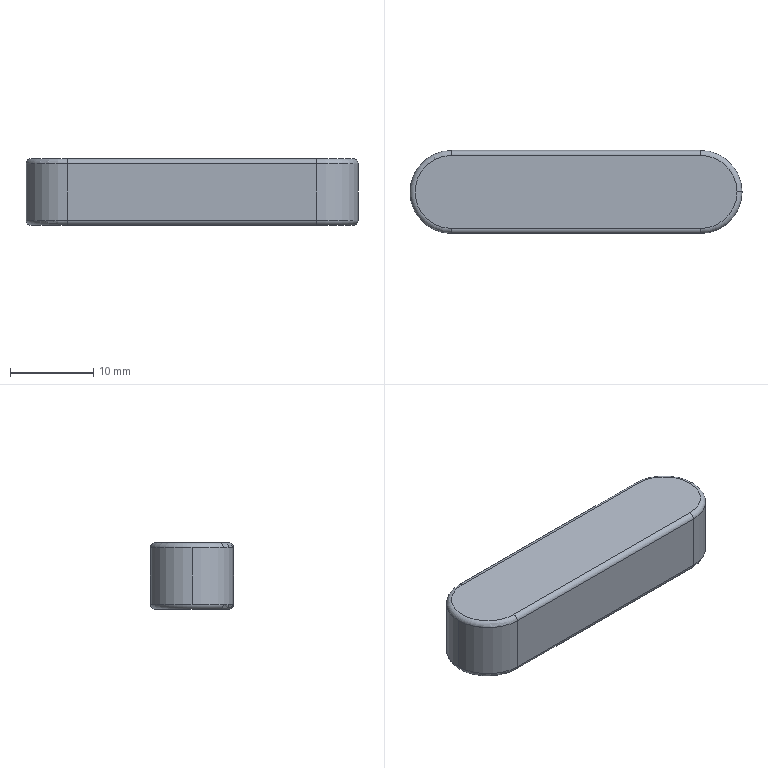Part | SolidWorks | features Extrusion 1, Fillet 1 | 1 solid | 17 faces | box 40 x 10 x 8 mm | volume 3014 mm3 | cylinder 7 | torus 6 | plane 4 | commonest cylinder face diameters 1.2 x4 10 x3
STEP:
#1=CARTESIAN_POINT('',(19.4,0.,0.));
#2=VERTEX_POINT('',#1);
#3=CARTESIAN_POINT('',(15.,-4.4,0.));
#4=VERTEX_POINT('',#3);
#5=CARTESIAN_POINT('',(15.,0.,0.));
#6=DIRECTION('',(0.,0.,-1.));
#7=DIRECTION('',(1.,0.,0.));
#8=AXIS2_PLACEMENT_3D('',#5,#6,#7);
#9=CIRCLE('',#8,4.4);
#10=EDGE_CURVE('',#2,#4,#9,.T.);
#11=ORIENTED_EDGE('',*,*,#10,.F.);
#12=CARTESIAN_POINT('',(20.,0.,0.6));
#13=VERTEX_POINT('',#12);
#14=CARTESIAN_POINT('',(19.4,0.,0.6));
#15=DIRECTION('',(0.,-1.,0.));
#16=DIRECTION('',(0.,0.,-1.));
#17=AXIS2_PLACEMENT_3D('',#14,#15,#16);
#18=CIRCLE('',#17,0.6);
#19=EDGE_CURVE('',#2,#13,#18,.T.);
#20=ORIENTED_EDGE('',*,*,#19,.T.);
#21=CARTESIAN_POINT('',(15.,-5.,0.6));
#22=VERTEX_POINT('',#21);
#23=CARTESIAN_POINT('',(15.,0.,0.6));
#24=DIRECTION('',(0.,0.,1.));
#25=DIRECTION('',(1.,0.,0.));
#26=AXIS2_PLACEMENT_3D('',#23,#24,#25);
#27=CIRCLE('',#26,5.);
#28=EDGE_CURVE('',#22,#13,#27,.T.);
#29=ORIENTED_EDGE('',*,*,#28,.F.);
#30=CARTESIAN_POINT('',(15.,-4.4,0.6));
#31=DIRECTION('',(1.,0.,0.));
#32=DIRECTION('',(0.,0.,-1.));
#33=AXIS2_PLACEMENT_3D('',#30,#31,#32);
#34=CIRCLE('',#33,0.6);
#35=EDGE_CURVE('',#22,#4,#34,.T.);
#36=ORIENTED_EDGE('',*,*,#35,.T.);
#37=EDGE_LOOP('',(#11,#20,#29,#36));
#38=FACE_OUTER_BOUND('',#37,.T.);
#39=CARTESIAN_POINT('',(15.,0.,0.6));
#40=DIRECTION('',(0.,0.,1.));
#41=DIRECTION('',(1.,0.,0.));
#42=AXIS2_PLACEMENT_3D('',#39,#40,#41);
#43=TOROIDAL_SURFACE('',#42,4.4,0.6);
#44=ADVANCED_FACE('',(#38),#43,.T.);
#45=CARTESIAN_POINT('',(20.,0.,7.4));
#46=VERTEX_POINT('',#45);
#47=CARTESIAN_POINT('',(15.,-5.,7.4));
#48=VERTEX_POINT('',#47);
#49=CARTESIAN_POINT('',(15.,0.,7.4));
#50=DIRECTION('',(0.,0.,-1.));
#51=DIRECTION('',(1.,0.,0.));
#52=AXIS2_PLACEMENT_3D('',#49,#50,#51);
#53=CIRCLE('',#52,5.);
#54=EDGE_CURVE('',#46,#48,#53,.T.);
#55=ORIENTED_EDGE('',*,*,#54,.F.);
#56=CARTESIAN_POINT('',(19.4,0.,8.));
#57=VERTEX_POINT('',#56);
#58=CARTESIAN_POINT('',(19.4,0.,7.4));
#59=DIRECTION('',(0.,-1.,0.));
#60=DIRECTION('',(0.,0.,-1.));
#61=AXIS2_PLACEMENT_3D('',#58,#59,#60);
#62=CIRCLE('',#61,0.6);
#63=EDGE_CURVE('',#46,#57,#62,.T.);
#64=ORIENTED_EDGE('',*,*,#63,.T.);
#65=CARTESIAN_POINT('',(15.,-4.4,8.));
#66=VERTEX_POINT('',#65);
#67=CARTESIAN_POINT('',(15.,0.,8.));
#68=DIRECTION('',(0.,0.,1.));
#69=DIRECTION('',(1.,0.,0.));
#70=AXIS2_PLACEMENT_3D('',#67,#68,#69);
#71=CIRCLE('',#70,4.4);
#72=EDGE_CURVE('',#66,#57,#71,.T.);
#73=ORIENTED_EDGE('',*,*,#72,.F.);
#74=CARTESIAN_POINT('',(15.,-4.4,7.4));
#75=DIRECTION('',(1.,0.,0.));
#76=DIRECTION('',(0.,0.,-1.));
#77=AXIS2_PLACEMENT_3D('',#74,#75,#76);
#78=CIRCLE('',#77,0.6);
#79=EDGE_CURVE('',#66,#48,#78,.T.);
#80=ORIENTED_EDGE('',*,*,#79,.T.);
#81=EDGE_LOOP('',(#55,#64,#73,#80));
#82=FACE_OUTER_BOUND('',#81,.T.);
#83=CARTESIAN_POINT('',(15.,0.,7.4));
#84=DIRECTION('',(0.,0.,1.));
#85=DIRECTION('',(1.,0.,0.));
#86=AXIS2_PLACEMENT_3D('',#83,#84,#85);
#87=TOROIDAL_SURFACE('',#86,4.4,0.6);
#88=ADVANCED_FACE('',(#82),#87,.T.);
#89=CARTESIAN_POINT('',(-15.,-5.,7.4));
#90=VERTEX_POINT('',#89);
#91=CARTESIAN_POINT('',(-20.,0.,7.4));
#92=VERTEX_POINT('',#91);
#93=CARTESIAN_POINT('',(-15.,0.,7.4));
#94=DIRECTION('',(0.,0.,-1.));
#95=DIRECTION('',(1.,0.,0.));
#96=AXIS2_PLACEMENT_3D('',#93,#94,#95);
#97=CIRCLE('',#96,5.);
#98=EDGE_CURVE('',#90,#92,#97,.T.);
#99=ORIENTED_EDGE('',*,*,#98,.T.);
#100=CARTESIAN_POINT('',(-20.,0.,0.6));
#101=VERTEX_POINT('',#100);
#102=CARTESIAN_POINT('',(-20.,0.,8.));
#103=DIRECTION('',(0.,0.,-1.));
#104=VECTOR('',#103,1000.);
#105=LINE('',#102,#104);
#106=EDGE_CURVE('',#92,#101,#105,.T.);
#107=ORIENTED_EDGE('',*,*,#106,.T.);
#108=CARTESIAN_POINT('',(-15.,-5.,0.6));
#109=VERTEX_POINT('',#108);
#110=CARTESIAN_POINT('',(-15.,0.,0.6));
#111=DIRECTION('',(0.,0.,1.));
#112=DIRECTION('',(1.,0.,0.));
#113=AXIS2_PLACEMENT_3D('',#110,#111,#112);
#114=CIRCLE('',#113,5.);
#115=EDGE_CURVE('',#101,#109,#114,.T.);
#116=ORIENTED_EDGE('',*,*,#115,.T.);
#117=CARTESIAN_POINT('',(-15.,-5.,8.));
#118=DIRECTION('',(0.,0.,-1.));
#119=VECTOR('',#118,1000.);
#120=LINE('',#117,#119);
#121=EDGE_CURVE('',#90,#109,#120,.T.);
#122=ORIENTED_EDGE('',*,*,#121,.F.);
#123=EDGE_LOOP('',(#99,#107,#116,#122));
#124=FACE_OUTER_BOUND('',#123,.T.);
#125=CARTESIAN_POINT('',(-15.,0.,8.));
#126=DIRECTION('',(0.,0.,-1.));
#127=DIRECTION('',(-1.,0.,0.));
#128=AXIS2_PLACEMENT_3D('',#125,#126,#127);
#129=CYLINDRICAL_SURFACE('',#128,5.);
#130=ADVANCED_FACE('',(#124),#129,.T.);
#131=ORIENTED_EDGE('',*,*,#106,.F.);
#132=CARTESIAN_POINT('',(-15.,5.,7.4));
#133=VERTEX_POINT('',#132);
#134=CARTESIAN_POINT('',(-15.,0.,7.4));
#135=DIRECTION('',(0.,0.,-1.));
#136=DIRECTION('',(1.,0.,0.));
#137=AXIS2_PLACEMENT_3D('',#134,#135,#136);
#138=CIRCLE('',#137,5.);
#139=EDGE_CURVE('',#92,#133,#138,.T.);
#140=ORIENTED_EDGE('',*,*,#139,.T.);
#141=CARTESIAN_POINT('',(-15.,5.,0.6));
#142=VERTEX_POINT('',#141);
#143=CARTESIAN_POINT('',(-15.,5.,8.));
#144=DIRECTION('',(0.,0.,-1.));
#145=VECTOR('',#144,1000.);
#146=LINE('',#143,#145);
#147=EDGE_CURVE('',#133,#142,#146,.T.);
#148=ORIENTED_EDGE('',*,*,#147,.T.);
#149=CARTESIAN_POINT('',(-15.,0.,0.6));
#150=DIRECTION('',(0.,0.,1.));
#151=DIRECTION('',(1.,0.,0.));
#152=AXIS2_PLACEMENT_3D('',#149,#150,#151);
#153=CIRCLE('',#152,5.);
#154=EDGE_CURVE('',#142,#101,#153,.T.);
#155=ORIENTED_EDGE('',*,*,#154,.T.);
#156=EDGE_LOOP('',(#131,#140,#148,#155));
#157=FACE_OUTER_BOUND('',#156,.T.);
#158=CARTESIAN_POINT('',(-15.,0.,8.));
#159=DIRECTION('',(0.,0.,-1.));
#160=DIRECTION('',(-1.,0.,0.));
#161=AXIS2_PLACEMENT_3D('',#158,#159,#160);
#162=CYLINDRICAL_SURFACE('',#161,5.);
#163=ADVANCED_FACE('',(#157),#162,.T.);
#164=CARTESIAN_POINT('',(15.,-5.,8.));
#165=DIRECTION('',(0.,0.,-1.));
#166=VECTOR('',#165,1000.);
#167=LINE('',#164,#166);
#168=EDGE_CURVE('',#48,#22,#167,.T.);
#169=ORIENTED_EDGE('',*,*,#168,.F.);
#170=CARTESIAN_POINT('',(-15.,-5.,7.4));
#171=DIRECTION('',(-1.,0.,0.));
#172=VECTOR('',#171,1000.);
#173=LINE('',#170,#172);
#174=EDGE_CURVE('',#48,#90,#173,.T.);
#175=ORIENTED_EDGE('',*,*,#174,.T.);
#176=ORIENTED_EDGE('',*,*,#121,.T.);
#177=CARTESIAN_POINT('',(-15.,-5.,0.6));
#178=DIRECTION('',(1.,0.,0.));
#179=VECTOR('',#178,1000.);
#180=LINE('',#177,#179);
#181=EDGE_CURVE('',#109,#22,#180,.T.);
#182=ORIENTED_EDGE('',*,*,#181,.T.);
#183=EDGE_LOOP('',(#169,#175,#176,#182));
#184=FACE_OUTER_BOUND('',#183,.T.);
#185=CARTESIAN_POINT('',(-15.,-5.,8.));
#186=DIRECTION('',(0.,1.,0.));
#187=DIRECTION('',(-1.,0.,0.));
#188=AXIS2_PLACEMENT_3D('',#185,#186,#187);
#189=PLANE('',#188);
#190=ADVANCED_FACE('',(#184),#189,.F.);
#191=CARTESIAN_POINT('',(15.,5.,7.4));
#192=VERTEX_POINT('',#191);
#193=CARTESIAN_POINT('',(15.,5.,0.6));
#194=VERTEX_POINT('',#193);
#195=CARTESIAN_POINT('',(15.,5.,8.));
#196=DIRECTION('',(0.,0.,-1.));
#197=VECTOR('',#196,1000.);
#198=LINE('',#195,#197);
#199=EDGE_CURVE('',#192,#194,#198,.T.);
#200=ORIENTED_EDGE('',*,*,#199,.F.);
#201=CARTESIAN_POINT('',(15.,0.,7.4));
#202=DIRECTION('',(0.,0.,-1.));
#203=DIRECTION('',(1.,0.,0.));
#204=AXIS2_PLACEMENT_3D('',#201,#202,#203);
#205=CIRCLE('',#204,5.);
#206=EDGE_CURVE('',#192,#46,#205,.T.);
#207=ORIENTED_EDGE('',*,*,#206,.T.);
#208=ORIENTED_EDGE('',*,*,#54,.T.);
#209=ORIENTED_EDGE('',*,*,#168,.T.);
#210=ORIENTED_EDGE('',*,*,#28,.T.);
#211=CARTESIAN_POINT('',(15.,0.,0.6));
#212=DIRECTION('',(0.,0.,1.));
#213=DIRECTION('',(1.,0.,0.));
#214=AXIS2_PLACEMENT_3D('',#211,#212,#213);
#215=CIRCLE('',#214,5.);
#216=EDGE_CURVE('',#13,#194,#215,.T.);
#217=ORIENTED_EDGE('',*,*,#216,.T.);
#218=EDGE_LOOP('',(#200,#207,#208,#209,#210,#217));
#219=FACE_OUTER_BOUND('',#218,.T.);
#220=CARTESIAN_POINT('',(15.,0.,8.));
#221=DIRECTION('',(0.,0.,-1.));
#222=DIRECTION('',(-1.,0.,0.));
#223=AXIS2_PLACEMENT_3D('',#220,#221,#222);
#224=CYLINDRICAL_SURFACE('',#223,5.);
#225=ADVANCED_FACE('',(#219),#224,.T.);
#226=ORIENTED_EDGE('',*,*,#147,.F.);
#227=CARTESIAN_POINT('',(15.,5.,7.4));
#228=DIRECTION('',(1.,0.,0.));
#229=VECTOR('',#228,1000.);
#230=LINE('',#227,#229);
#231=EDGE_CURVE('',#133,#192,#230,.T.);
#232=ORIENTED_EDGE('',*,*,#231,.T.);
#233=ORIENTED_EDGE('',*,*,#199,.T.);
#234=CARTESIAN_POINT('',(-15.,5.,0.6));
#235=DIRECTION('',(-1.,0.,0.));
#236=VECTOR('',#235,1000.);
#237=LINE('',#234,#236);
#238=EDGE_CURVE('',#194,#142,#237,.T.);
#239=ORIENTED_EDGE('',*,*,#238,.T.);
#240=EDGE_LOOP('',(#226,#232,#233,#239));
#241=FACE_OUTER_BOUND('',#240,.T.);
#242=CARTESIAN_POINT('',(-15.,5.,8.));
#243=DIRECTION('',(0.,-1.,0.));
#244=DIRECTION('',(1.,0.,0.));
#245=AXIS2_PLACEMENT_3D('',#242,#243,#244);
#246=PLANE('',#245);
#247=ADVANCED_FACE('',(#241),#246,.F.);
#248=CARTESIAN_POINT('',(-15.,-4.4,8.));
#249=VERTEX_POINT('',#248);
#250=CARTESIAN_POINT('',(15.,-4.4,8.));
#251=DIRECTION('',(1.,0.,0.));
#252=VECTOR('',#251,1000.);
#253=LINE('',#250,#252);
#254=EDGE_CURVE('',#249,#66,#253,.T.);
#255=ORIENTED_EDGE('',*,*,#254,.T.);
#256=ORIENTED_EDGE('',*,*,#72,.T.);
#257=CARTESIAN_POINT('',(15.,4.4,8.));
#258=VERTEX_POINT('',#257);
#259=CARTESIAN_POINT('',(15.,0.,8.));
#260=DIRECTION('',(0.,0.,1.));
#261=DIRECTION('',(1.,0.,0.));
#262=AXIS2_PLACEMENT_3D('',#259,#260,#261);
#263=CIRCLE('',#262,4.4);
#264=EDGE_CURVE('',#57,#258,#263,.T.);
#265=ORIENTED_EDGE('',*,*,#264,.T.);
#266=CARTESIAN_POINT('',(-15.,4.4,8.));
#267=VERTEX_POINT('',#266);
#268=CARTESIAN_POINT('',(-15.,4.4,8.));
#269=DIRECTION('',(-1.,0.,0.));
#270=VECTOR('',#269,1000.);
#271=LINE('',#268,#270);
#272=EDGE_CURVE('',#258,#267,#271,.T.);
#273=ORIENTED_EDGE('',*,*,#272,.T.);
#274=CARTESIAN_POINT('',(-15.,0.,8.));
#275=DIRECTION('',(0.,0.,1.));
#276=DIRECTION('',(1.,0.,0.));
#277=AXIS2_PLACEMENT_3D('',#274,#275,#276);
#278=CIRCLE('',#277,4.4);
#279=EDGE_CURVE('',#267,#249,#278,.T.);
#280=ORIENTED_EDGE('',*,*,#279,.T.);
#281=EDGE_LOOP('',(#255,#256,#265,#273,#280));
#282=FACE_OUTER_BOUND('',#281,.T.);
#283=CARTESIAN_POINT('',(-15.,0.,8.));
#284=DIRECTION('',(0.,0.,1.));
#285=DIRECTION('',(1.,0.,0.));
#286=AXIS2_PLACEMENT_3D('',#283,#284,#285);
#287=PLANE('',#286);
#288=ADVANCED_FACE('',(#282),#287,.T.);
#289=CARTESIAN_POINT('',(-15.,4.4,0.));
#290=VERTEX_POINT('',#289);
#291=CARTESIAN_POINT('',(15.,4.4,0.));
#292=VERTEX_POINT('',#291);
#293=CARTESIAN_POINT('',(-15.,4.4,0.));
#294=DIRECTION('',(1.,0.,0.));
#295=VECTOR('',#294,1000.);
#296=LINE('',#293,#295);
#297=EDGE_CURVE('',#290,#292,#296,.T.);
#298=ORIENTED_EDGE('',*,*,#297,.T.);
#299=CARTESIAN_POINT('',(15.,0.,0.));
#300=DIRECTION('',(0.,0.,-1.));
#301=DIRECTION('',(1.,0.,0.));
#302=AXIS2_PLACEMENT_3D('',#299,#300,#301);
#303=CIRCLE('',#302,4.4);
#304=EDGE_CURVE('',#292,#2,#303,.T.);
#305=ORIENTED_EDGE('',*,*,#304,.T.);
#306=ORIENTED_EDGE('',*,*,#10,.T.);
#307=CARTESIAN_POINT('',(-15.,-4.4,0.));
#308=VERTEX_POINT('',#307);
#309=CARTESIAN_POINT('',(-15.,-4.4,0.));
#310=DIRECTION('',(-1.,0.,0.));
#311=VECTOR('',#310,1000.);
#312=LINE('',#309,#311);
#313=EDGE_CURVE('',#4,#308,#312,.T.);
#314=ORIENTED_EDGE('',*,*,#313,.T.);
#315=CARTESIAN_POINT('',(-15.,0.,0.));
#316=DIRECTION('',(0.,0.,-1.));
#317=DIRECTION('',(1.,0.,0.));
#318=AXIS2_PLACEMENT_3D('',#315,#316,#317);
#319=CIRCLE('',#318,4.4);
#320=EDGE_CURVE('',#308,#290,#319,.T.);
#321=ORIENTED_EDGE('',*,*,#320,.T.);
#322=EDGE_LOOP('',(#298,#305,#306,#314,#321));
#323=FACE_OUTER_BOUND('',#322,.T.);
#324=CARTESIAN_POINT('',(-15.,0.,0.));
#325=DIRECTION('',(0.,0.,1.));
#326=DIRECTION('',(1.,0.,0.));
#327=AXIS2_PLACEMENT_3D('',#324,#325,#326);
#328=PLANE('',#327);
#329=ADVANCED_FACE('',(#323),#328,.F.);
#330=CARTESIAN_POINT('',(-15.,4.4,7.4));
#331=DIRECTION('',(1.,0.,0.));
#332=DIRECTION('',(0.,0.,-1.));
#333=AXIS2_PLACEMENT_3D('',#330,#331,#332);
#334=CIRCLE('',#333,0.6);
#335=EDGE_CURVE('',#133,#267,#334,.T.);
#336=ORIENTED_EDGE('',*,*,#335,.F.);
#337=ORIENTED_EDGE('',*,*,#139,.F.);
#338=ORIENTED_EDGE('',*,*,#98,.F.);
#339=CARTESIAN_POINT('',(-15.,-4.4,7.4));
#340=DIRECTION('',(1.,0.,0.));
#341=DIRECTION('',(0.,0.,-1.));
#342=AXIS2_PLACEMENT_3D('',#339,#340,#341);
#343=CIRCLE('',#342,0.6);
#344=EDGE_CURVE('',#249,#90,#343,.T.);
#345=ORIENTED_EDGE('',*,*,#344,.F.);
#346=ORIENTED_EDGE('',*,*,#279,.F.);
#347=EDGE_LOOP('',(#336,#337,#338,#345,#346));
#348=FACE_OUTER_BOUND('',#347,.T.);
#349=CARTESIAN_POINT('',(-15.,0.,7.4));
#350=DIRECTION('',(0.,0.,1.));
#351=DIRECTION('',(1.,0.,0.));
#352=AXIS2_PLACEMENT_3D('',#349,#350,#351);
#353=TOROIDAL_SURFACE('',#352,4.4,0.6);
#354=ADVANCED_FACE('',(#348),#353,.T.);
#355=ORIENTED_EDGE('',*,*,#344,.T.);
#356=ORIENTED_EDGE('',*,*,#174,.F.);
#357=ORIENTED_EDGE('',*,*,#79,.F.);
#358=ORIENTED_EDGE('',*,*,#254,.F.);
#359=EDGE_LOOP('',(#355,#356,#357,#358));
#360=FACE_OUTER_BOUND('',#359,.T.);
#361=CARTESIAN_POINT('',(-15.,-4.4,7.4));
#362=DIRECTION('',(-1.,0.,0.));
#363=DIRECTION('',(0.,-1.,0.));
#364=AXIS2_PLACEMENT_3D('',#361,#362,#363);
#365=CYLINDRICAL_SURFACE('',#364,0.6);
#366=ADVANCED_FACE('',(#360),#365,.T.);
#367=ORIENTED_EDGE('',*,*,#335,.T.);
#368=ORIENTED_EDGE('',*,*,#272,.F.);
#369=CARTESIAN_POINT('',(15.,4.4,7.4));
#370=DIRECTION('',(1.,0.,0.));
#371=DIRECTION('',(0.,0.,-1.));
#372=AXIS2_PLACEMENT_3D('',#369,#370,#371);
#373=CIRCLE('',#372,0.6);
#374=EDGE_CURVE('',#192,#258,#373,.T.);
#375=ORIENTED_EDGE('',*,*,#374,.F.);
#376=ORIENTED_EDGE('',*,*,#231,.F.);
#377=EDGE_LOOP('',(#367,#368,#375,#376));
#378=FACE_OUTER_BOUND('',#377,.T.);
#379=CARTESIAN_POINT('',(-15.,4.4,7.4));
#380=DIRECTION('',(1.,0.,0.));
#381=DIRECTION('',(0.,1.,0.));
#382=AXIS2_PLACEMENT_3D('',#379,#380,#381);
#383=CYLINDRICAL_SURFACE('',#382,0.6);
#384=ADVANCED_FACE('',(#378),#383,.T.);
#385=ORIENTED_EDGE('',*,*,#63,.F.);
#386=ORIENTED_EDGE('',*,*,#206,.F.);
#387=ORIENTED_EDGE('',*,*,#374,.T.);
#388=ORIENTED_EDGE('',*,*,#264,.F.);
#389=EDGE_LOOP('',(#385,#386,#387,#388));
#390=FACE_OUTER_BOUND('',#389,.T.);
#391=CARTESIAN_POINT('',(15.,0.,7.4));
#392=DIRECTION('',(0.,0.,1.));
#393=DIRECTION('',(1.,0.,0.));
#394=AXIS2_PLACEMENT_3D('',#391,#392,#393);
#395=TOROIDAL_SURFACE('',#394,4.4,0.6);
#396=ADVANCED_FACE('',(#390),#395,.T.);
#397=CARTESIAN_POINT('',(-15.,4.4,0.6));
#398=DIRECTION('',(1.,0.,0.));
#399=DIRECTION('',(0.,0.,-1.));
#400=AXIS2_PLACEMENT_3D('',#397,#398,#399);
#401=CIRCLE('',#400,0.6);
#402=EDGE_CURVE('',#290,#142,#401,.T.);
#403=ORIENTED_EDGE('',*,*,#402,.F.);
#404=ORIENTED_EDGE('',*,*,#320,.F.);
#405=CARTESIAN_POINT('',(-15.,-4.4,0.6));
#406=DIRECTION('',(1.,0.,0.));
#407=DIRECTION('',(0.,0.,-1.));
#408=AXIS2_PLACEMENT_3D('',#405,#406,#407);
#409=CIRCLE('',#408,0.6);
#410=EDGE_CURVE('',#109,#308,#409,.T.);
#411=ORIENTED_EDGE('',*,*,#410,.F.);
#412=ORIENTED_EDGE('',*,*,#115,.F.);
#413=ORIENTED_EDGE('',*,*,#154,.F.);
#414=EDGE_LOOP('',(#403,#404,#411,#412,#413));
#415=FACE_OUTER_BOUND('',#414,.T.);
#416=CARTESIAN_POINT('',(-15.,0.,0.6));
#417=DIRECTION('',(0.,0.,1.));
#418=DIRECTION('',(1.,0.,0.));
#419=AXIS2_PLACEMENT_3D('',#416,#417,#418);
#420=TOROIDAL_SURFACE('',#419,4.4,0.6);
#421=ADVANCED_FACE('',(#415),#420,.T.);
#422=ORIENTED_EDGE('',*,*,#410,.T.);
#423=ORIENTED_EDGE('',*,*,#313,.F.);
#424=ORIENTED_EDGE('',*,*,#35,.F.);
#425=ORIENTED_EDGE('',*,*,#181,.F.);
#426=EDGE_LOOP('',(#422,#423,#424,#425));
#427=FACE_OUTER_BOUND('',#426,.T.);
#428=CARTESIAN_POINT('',(-15.,-4.4,0.6));
#429=DIRECTION('',(1.,0.,0.));
#430=DIRECTION('',(0.,1.,0.));
#431=AXIS2_PLACEMENT_3D('',#428,#429,#430);
#432=CYLINDRICAL_SURFACE('',#431,0.6);
#433=ADVANCED_FACE('',(#427),#432,.T.);
#434=ORIENTED_EDGE('',*,*,#402,.T.);
#435=ORIENTED_EDGE('',*,*,#238,.F.);
#436=CARTESIAN_POINT('',(15.,4.4,0.6));
#437=DIRECTION('',(1.,0.,0.));
#438=DIRECTION('',(0.,0.,-1.));
#439=AXIS2_PLACEMENT_3D('',#436,#437,#438);
#440=CIRCLE('',#439,0.6);
#441=EDGE_CURVE('',#292,#194,#440,.T.);
#442=ORIENTED_EDGE('',*,*,#441,.F.);
#443=ORIENTED_EDGE('',*,*,#297,.F.);
#444=EDGE_LOOP('',(#434,#435,#442,#443));
#445=FACE_OUTER_BOUND('',#444,.T.);
#446=CARTESIAN_POINT('',(-15.,4.4,0.6));
#447=DIRECTION('',(-1.,0.,0.));
#448=DIRECTION('',(0.,-1.,0.));
#449=AXIS2_PLACEMENT_3D('',#446,#447,#448);
#450=CYLINDRICAL_SURFACE('',#449,0.6);
#451=ADVANCED_FACE('',(#445),#450,.T.);
#452=ORIENTED_EDGE('',*,*,#19,.F.);
#453=ORIENTED_EDGE('',*,*,#304,.F.);
#454=ORIENTED_EDGE('',*,*,#441,.T.);
#455=ORIENTED_EDGE('',*,*,#216,.F.);
#456=EDGE_LOOP('',(#452,#453,#454,#455));
#457=FACE_OUTER_BOUND('',#456,.T.);
#458=CARTESIAN_POINT('',(15.,0.,0.6));
#459=DIRECTION('',(0.,0.,1.));
#460=DIRECTION('',(1.,0.,0.));
#461=AXIS2_PLACEMENT_3D('',#458,#459,#460);
#462=TOROIDAL_SURFACE('',#461,4.4,0.6);
#463=ADVANCED_FACE('',(#457),#462,.T.);
#464=CLOSED_SHELL('',(#44,#88,#130,#163,#190,#225,#247,#288,#329,#354,#366,#384,#396,#421,#433,#451,#463));
#465=MANIFOLD_SOLID_BREP('',#464);
#466=CARTESIAN_POINT('',(0.,0.,0.));
#467=DIRECTION('',(0.,0.,1.));
#468=DIRECTION('',(1.,0.,0.));
#469=AXIS2_PLACEMENT_3D('',#466,#467,#468);
#470=(LENGTH_UNIT()NAMED_UNIT(*)SI_UNIT(.MILLI.,.METRE.));
#471=UNCERTAINTY_MEASURE_WITH_UNIT(LENGTH_MEASURE(0.00001),#470,'','');
#472=(NAMED_UNIT(*)PLANE_ANGLE_UNIT()SI_UNIT($,.RADIAN.));
#473=(NAMED_UNIT(*)SI_UNIT($,.STERADIAN.)SOLID_ANGLE_UNIT());
#474=(GEOMETRIC_REPRESENTATION_CONTEXT(3)GLOBAL_UNCERTAINTY_ASSIGNED_CONTEXT((#471))GLOBAL_UNIT_ASSIGNED_CONTEXT((#470,#472,#473))REPRESENTATION_CONTEXT('',''));
#475=ADVANCED_BREP_SHAPE_REPRESENTATION('',(#465,#469),#474);